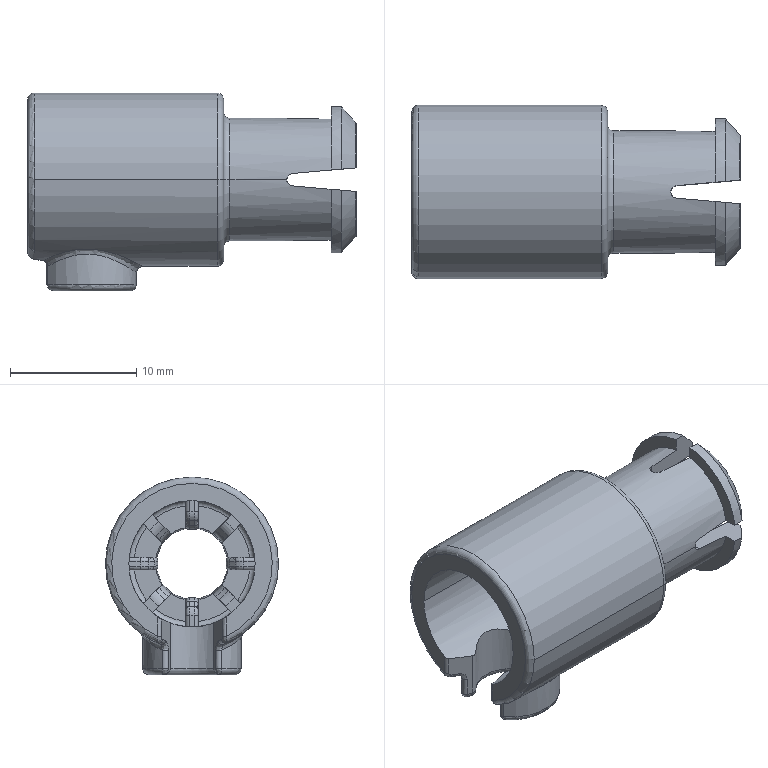Part | STEP file | MSBR-23 | 1 solid | 212 faces | box 26 x 13.7 x 15.65 mm | volume 1729 mm3 | plane 69 | torus 57 | cylinder 52 | cone 16 | spline 16 | sphere 2 | commonest cylinder face diameters 0.6 x20 1 x8 7 x8 5.4 x4 11.7 x4 9.7 x2